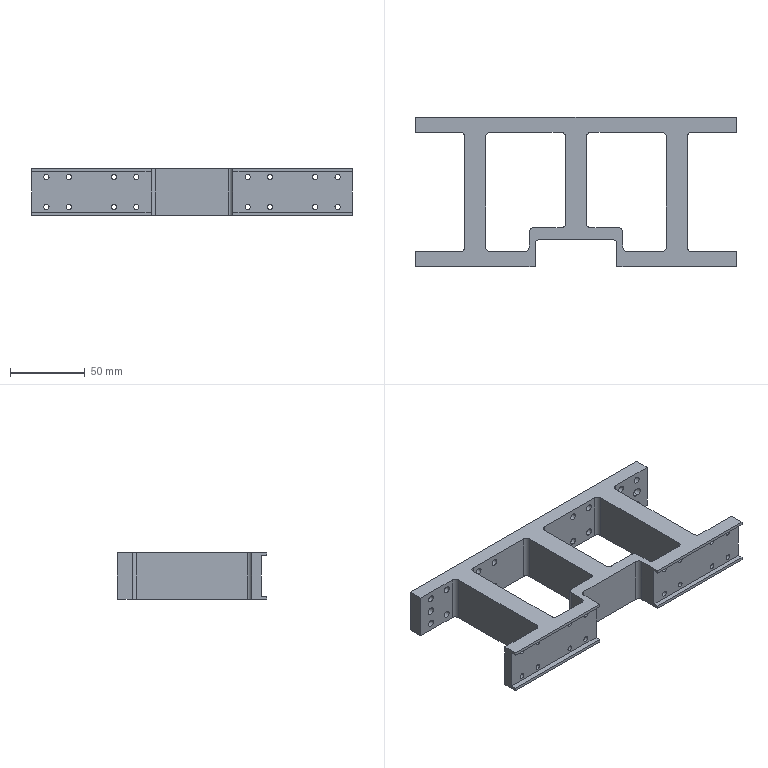CAM job | NX | 3-axis milling | part box 215 x 100 x 31 mm | stock box 221 x 102 x 32 mm
Tools:
number,name,description,diameter,corner_radius,flute_length,length,flutes
1,D63,Milling Tool-5 Parameters,63.0,0.0,50.0,75.0,2
10,D10,Milling Tool-5 Parameters,10.0,0.0,50.0,75.0,2
11,D10JING,Milling Tool-5 Parameters,10.0,0.0,50.0,75.0,2
7,D6A45,Milling Tool-5 Parameters,6.0,0.0,3.0,3.0,2
6,D6,Milling Tool-5 Parameters,6.0,0.0,50.0,75.0,2
Operations:
program,operation,operation_type,tool,method,geometry_group,spindle_rpm,surface_speed,feed_per_tooth,feed_cut,feed_plunge,cut_length_mm,path_length_mm,cut_time_min,machine_time_min
1-218-100-35毛胚,FLOOR_WALL,VolumeBased25DMillingOperation,D63,METHOD,A,6500.0,1286.0,0.0962,1250.0,100.0,940.797,994.797,0.7526,0.758
1-218-100-35毛胚,ADAPTIVE_MILLING,CavityMilling,D10,METHOD,A,7000.0,219.0,0.2143,3000.0,1000.0,68216.652,70033.013,25.578,25.759
1-218-100-35毛胚,ZLEVEL_PROFILE_COPY_COPY_1,ZLevelMilling,D10JING,METHOD,A,7000.0,219.0,0.0714,1000.0,100.0,2597.803,3209.398,2.598,2.659
1-218-100-35毛胚,ZLEVEL_PROFILE_COPY_1,ZLevelMilling,D6,METHOD,A,7000.0,131.0,0.0857,1200.0,1000.0,7705.904,12920.252,6.697,7.219
1-218-100-35毛胚,ZLEVEL_PROFILE_COPY_1_COPY_COPY_COPY_COPY_2_COPY,ZLevelMilling,D6A45,METHOD,A,7000.0,131.0,0.0714,1000.0,1000.0,1312.436,1824.667,1.312,1.364